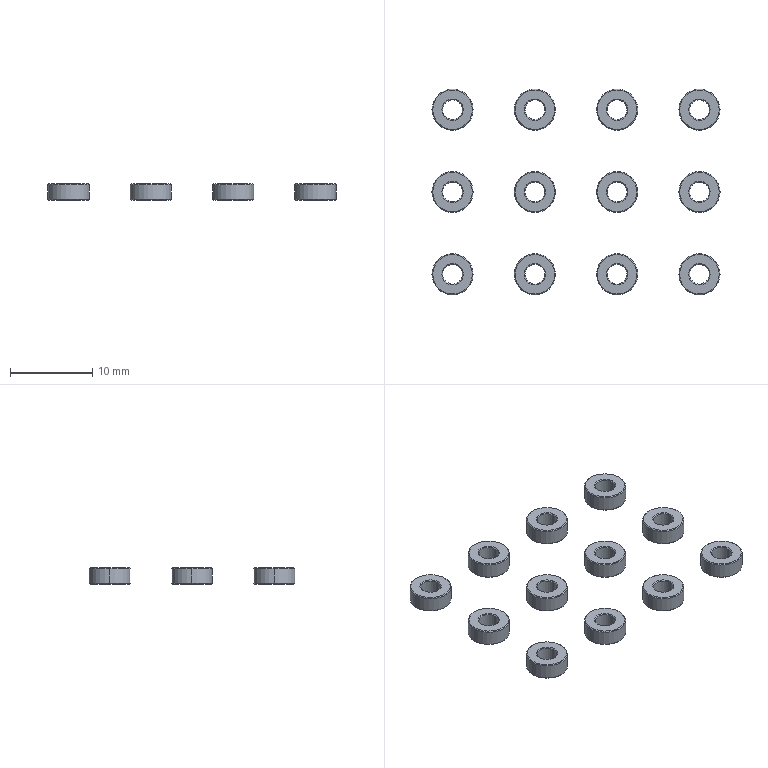NC program | NX | posted with a generic post | part box 35 x 25 x 2 mm
Lines 3718 to 5177 of 5177:
(ZLEVEL_PROFILE_1_COPY , TOOL : D6A45)
N7422 T07 M6
N7424 G54
N7426 G17 G0 G90 X2.2 Y22.5 S9500 M3
N7428 G43 Z30. H7
N7430 Z2.
N7432 G94 G1 Z-1. F1250.
N7434 G3 X2.5 Y22.2 R0.3
N7436 X2.2 Y22.5 R-0.3
N7438 X2.35 Y22.24 R0.3
N7440 G1 Z1.
N7442 G0 Z30.
N7444 X32.5 Y22.8
N7446 Z2.
N7448 G1 Z-1.
N7450 G3 X32.2 Y22.5 R0.3
N7452 X32.5 Y22.8 R-0.3
N7454 X32.24 Y22.65 R0.3
N7456 G1 Z1.
N7458 G0 Z30.
N7460 X22.5 Y22.8
N7462 Z2.
N7464 G1 Z-1.
N7466 G3 X22.2 Y22.5 R0.3
N7468 X22.5 Y22.8 R-0.3
N7470 X22.24 Y22.65 R0.3
N7472 G1 Z1.
N7474 G0 Z30.
N7476 X12.5 Y22.8
N7478 Z2.
N7480 G1 Z-1.
N7482 G3 X12.2 Y22.5 R0.3
N7484 X12.5 Y22.8 R-0.3
N7486 X12.24 Y22.65 R0.3
N7488 G1 Z1.
N7490 G0 Z30.
N7492 X32.8 Y12.5
N7494 Z2.
N7496 G1 Z-1.
N7498 Y12.512
N7500 G3 X32.8 Y12.5 R-0.3
N7502 X32.65 Y12.76 R0.3
N7504 G1 Z1.
N7506 G0 Z30.
N7508 X22.5 Y12.8
N7510 Z2.
N7512 G1 Z-1.
N7514 G3 X22.2 Y12.5 R0.3
N7516 X22.5 Y12.8 R-0.3
N7518 X22.24 Y12.65 R0.3
N7520 G1 Z1.
N7522 G0 Z30.
N7524 X12.5 Y12.2
N7526 Z2.
N7528 G1 Z-1.
N7530 G3 X12.8 Y12.5 R0.3
N7532 X12.5 Y12.2 R-0.3
N7534 X12.76 Y12.35 R0.3
N7536 G1 Z1.
N7538 G0 Z30.
N7540 X2.2 Y12.5
N7542 Z2.
N7544 G1 Z-1.
N7546 Y12.488
N7548 G3 X2.2 Y12.5 R-0.3
N7550 X2.35 Y12.24 R0.3
N7552 G1 Z1.
N7554 G0 Z30.
N7556 X32.5 Y2.2
N7558 Z2.
N7560 G1 Z-1.
N7562 G3 X32.8 Y2.5 R0.3
N7564 X32.5 Y2.2 R-0.3
N7566 X32.76 Y2.35 R0.3
N7568 G1 Z1.
N7570 G0 Z30.
N7572 X22.5 Y2.2
N7574 Z2.
N7576 G1 Z-1.
N7578 X22.553 Y2.205
N7580 G3 X22.5 Y2.2 R-0.3
N7582 X22.76 Y2.35 R0.3
N7584 G1 Z1.
N7586 G0 Z30.
N7588 X12.5 Y2.2
N7590 Z2.
N7592 G1 Z-1.
N7594 G3 X12.8 Y2.5 R0.3
N7596 X12.5 Y2.2 R-0.3
N7598 X12.76 Y2.35 R0.3
N7600 G1 Z1.
N7602 G0 Z30.
N7604 X2.5 Y2.2
N7606 Z2.
N7608 G1 Z-1.
N7610 G3 X2.8 Y2.5 R0.3
N7612 X2.5 Y2.2 R-0.3
N7614 X2.76 Y2.35 R0.3
N7616 G1 Z1.
N7618 G0 Z30.
N7620 X3.478 Y-1.995
N7622 Z1.
N7624 G1 Z-1.
N7626 X3.02 Y-1.2
N7628 G3 X2.5 Y-0.9 R0.6
N7630 G2 X-0.9 Y2.5 R3.4
N7632 X2.5 Y-0.9 R-3.4
N7634 G3 X1.98 Y-1.2 R0.6
N7636 G1 X1.522 Y-1.995
N7638 Z1.
N7640 G0 Z30.
N7642 X13.478
N7644 Z1.
N7646 G1 Z-1.
N7648 X13.02 Y-1.2
N7650 G3 X12.5 Y-0.9 R0.6
N7652 G2 X9.1 Y2.5 R3.4
N7654 X12.5 Y-0.9 R-3.4
N7656 G3 X11.98 Y-1.2 R0.6
N7658 G1 X11.522 Y-1.995
N7660 Z1.
N7662 G0 Z30.
N7664 X23.478
N7666 Z1.
N7668 G1 Z-1.
N7670 X23.02 Y-1.2
N7672 G3 X22.5 Y-0.9 R0.6
N7674 G2 X19.1 Y2.5 R3.4
N7676 X22.5 Y-0.9 R-3.4
N7678 G3 X21.98 Y-1.2 R0.6
N7680 G1 X21.522 Y-1.995
N7682 Z1.
N7684 G0 Z30.
N7686 X33.478
N7688 Z1.
N7690 G1 Z-1.
N7692 X33.02 Y-1.2
N7694 G3 X32.5 Y-0.9 R0.6
N7696 G2 X29.1 Y2.5 R3.4
N7698 X32.5 Y-0.9 R-3.4
N7700 G3 X31.98 Y-1.2 R0.6
N7702 G1 X31.522 Y-1.995
N7704 Z1.
N7706 G0 Z30.
N7708 X-1.995 Y11.522
N7710 Z1.
N7712 G1 Z-1.
N7714 X-1.2 Y11.98
N7716 G3 X-0.9 Y12.5 R0.6
N7718 G1 Y12.504
N7720 G2 X2.504 Y15.9 R3.4
N7722 X-0.9 Y12.5 R-3.4
N7724 G3 X-1.2 Y13.02 R0.6
N7726 G1 X-1.995 Y13.478
N7728 Z1.
N7730 G0 Z30.
N7732 X8.005 Y11.522
N7734 Z1.
N7736 G1 Z-1.
N7738 X8.8 Y11.98
N7740 G3 X9.1 Y12.5 R0.6
N7742 G2 X12.5 Y15.9 R3.4
N7744 X9.1 Y12.5 R-3.4
N7746 G3 X8.8 Y13.02 R0.6
N7748 G1 X8.005 Y13.478
N7750 Z1.
N7752 G0 Z30.
N7754 X21.522 Y16.995
N7756 Z1.
N7758 G1 Z-1.
N7760 X21.98 Y16.2
N7762 G3 X22.5 Y15.9 R0.6
N7764 G2 X25.9 Y12.5 R3.4
N7766 X22.5 Y15.9 R-3.4
N7768 G3 X23.02 Y16.2 R0.6
N7770 G1 X23.478 Y16.995
N7772 Z1.
N7774 G0 Z30.
N7776 X36.995 Y13.478
N7778 Z1.
N7780 G1 Z-1.
N7782 X36.2 Y13.02
N7784 G3 X35.9 Y12.5 R0.6
N7786 G1 Y12.496
N7788 G2 X32.496 Y9.1 R3.4
N7790 X35.9 Y12.5 R-3.4
N7792 G3 X36.2 Y11.98 R0.6
N7794 G1 X36.995 Y11.522
N7796 Z1.
N7798 G0 Z30.
N7800 X11.522 Y26.995
N7802 Z1.
N7804 G1 Z-1.
N7806 X11.98 Y26.2
N7808 G3 X12.5 Y25.9 R0.6
N7810 G2 X15.9 Y22.5 R3.4
N7812 X12.5 Y25.9 R-3.4
N7814 G3 X13.02 Y26.2 R0.6
N7816 G1 X13.478 Y26.995
N7818 Z1.
N7820 G0 Z30.
N7822 X21.522
N7824 Z1.
N7826 G1 Z-1.
N7828 X21.98 Y26.2
N7830 G3 X22.5 Y25.9 R0.6
N7832 G2 X25.9 Y22.5 R3.4
N7834 X22.5 Y25.9 R-3.4
N7836 G3 X23.02 Y26.2 R0.6
N7838 G1 X23.478 Y26.995
N7840 Z1.
N7842 G0 Z30.
N7844 X31.522
N7846 Z1.
N7848 G1 Z-1.
N7850 X31.98 Y26.2
N7852 G3 X32.5 Y25.9 R0.6
N7854 G2 X35.9 Y22.5 R3.4
N7856 X32.5 Y25.9 R-3.4
N7858 G3 X33.02 Y26.2 R0.6
N7860 G1 X33.478 Y26.995
N7862 Z1.
N7864 G0 Z30.
N7866 X1.522
N7868 Z1.
N7870 G1 Z-1.
N7872 X1.98 Y26.2
N7874 G3 X2.5 Y25.9 R0.6
N7876 G2 X5.9 Y22.5 R3.4
N7878 X2.5 Y25.9 R-3.4
N7880 G3 X3.02 Y26.2 R0.6
N7882 G1 X3.478 Y26.995
N7884 Z1.
N7886 G0 Z30.
N7888 M5
(ZLEVEL_PROFILE_COPY , TOOL : D4)
N7890 T04 M6
N7892 G54
N7894 G17 G0 G90 X36.171 Y15.114 S9500 M3
N7896 G43 Z30. H4
N7898 Z0.1
N7900 G94 G1 X36.688 Y14.227 Z0.046 F1000.
N7902 X36.998 Y13.036 Z-0.018
N7904 X37. Y12.5 Z-0.046
N7906 Y11.98 Z-0.074
N7908 X36.848 Y11.229 Z-0.114
N7910 X36.572 Y10.514 Z-0.154
N7912 X36.011 Y9.637 Z-0.208
N7914 X35.025 Y8.739 Z-0.278
N7916 X33.82 Y8.166 Z-0.348
N7918 X32.5 Y7.97 Z-0.418
N7920 X31.18 Y8.166 Z-0.488
N7922 X29.975 Y8.739 Z-0.558
N7924 X28.989 Y9.637 Z-0.628
N7926 X28.428 Y10.514 Z-0.683
N7928 X28.15 Y11.236 Z-0.723
N7930 X27.998 Y11.995 Z-0.764
N7932 X28.002 Y13.036 Z-0.818
N7934 X28.392 Y14.41 Z-0.893
N7936 X29.192 Y15.595 Z-0.968
N7938 X30.321 Y16.471 Z-1.043
N7940 X31.666 Y16.953 Z-1.118
N7942 X33.095 Y16.991 Z-1.193
N7944 X34.104 Y16.737 Z-1.247
N7946 X35.185 Y16.148 Z-1.312
N7948 X36.068 Y15.291 Z-1.376
N7950 X36.688 Y14.227 Z-1.441
N7952 X36.998 Y13.036 Z-1.505
N7954 X37. Y12.5 Z-1.533
N7956 G2 X32.5 Y8. R4.5
N7958 X37. Y12.5 R-4.5
N7960 G1 X36.994 Y12.261 Z-1.538
N7962 X36.975 Y12.023 Z-1.542
N7964 X36.943 Y11.787 Z-1.546
N7966 X36.899 Y11.552 Z-1.55
N7968 X36.843 Y11.32 Z-1.554
N7970 X36.774 Y11.092 Z-1.558
N7972 X36.693 Y10.867 Z-1.563
N7974 X36.601 Y10.647 Z-1.567
N7976 X36.497 Y10.432 Z-1.571
N7978 X36.382 Y10.223 Z-1.575
N7980 X36.255 Y10.021 Z-1.579
N7982 X36.119 Y9.825 Z-1.583
N7984 X35.972 Y9.637 Z-1.588
N7986 X35.815 Y9.457 Z-1.592
N7988 X35.649 Y9.285 Z-1.596
N7990 X35.474 Y9.123 Z-1.6
N7992 X35.291 Y8.97 Z-1.604
N7994 X35.1 Y8.827 Z-1.608
N7996 X34.901 Y8.694 Z-1.613
N7998 X34.696 Y8.572 Z-1.617
N8000 X34.485 Y8.461 Z-1.621
N8002 X34.268 Y8.362 Z-1.625
N8004 X34.046 Y8.274 Z-1.629
N8006 X33.82 Y8.198 Z-1.633
N8008 X33.59 Y8.134 Z-1.638
N8010 X33.357 Y8.082 Z-1.642
N8012 X33.121 Y8.043 Z-1.646
N8014 X32.884 Y8.016 Z-1.65
N8016 X32.646 Y8.002 Z-1.654
N8018 X32.407 Y8.001 Z-1.658
N8020 X32.169 Y8.012 Z-1.663
N8022 X31.931 Y8.036 Z-1.667
N8024 G2 X37. Y12.5 R-4.5
N8026 G1 X36.994 Y12.261 Z-1.671
N8028 X36.975 Y12.023 Z-1.675
N8030 X36.943 Y11.787 Z-1.679
N8032 X36.899 Y11.552 Z-1.683
N8034 X36.843 Y11.32 Z-1.688
N8036 X36.774 Y11.092 Z-1.692
N8038 X36.693 Y10.867 Z-1.696
N8040 X36.601 Y10.647 Z-1.7
N8042 X36.497 Y10.432 Z-1.704
N8044 X36.382 Y10.223 Z-1.708
N8046 X36.255 Y10.021 Z-1.713
N8048 X36.119 Y9.825 Z-1.717
N8050 X35.972 Y9.637 Z-1.721
N8052 X35.815 Y9.457 Z-1.725
N8054 X35.649 Y9.285 Z-1.729
N8056 X35.474 Y9.123 Z-1.733
N8058 X35.291 Y8.97 Z-1.738
N8060 X35.1 Y8.827 Z-1.742
N8062 X34.901 Y8.694 Z-1.746
N8064 X34.696 Y8.572 Z-1.75
N8066 X34.485 Y8.461 Z-1.754
N8068 X34.268 Y8.362 Z-1.758
N8070 X34.046 Y8.274 Z-1.763
N8072 X33.82 Y8.198 Z-1.767
N8074 X33.59 Y8.134 Z-1.771
N8076 X33.357 Y8.082 Z-1.775
N8078 X33.121 Y8.043 Z-1.779
N8080 X32.884 Y8.016 Z-1.783
N8082 X32.646 Y8.002 Z-1.788
N8084 X32.407 Y8.001 Z-1.792
N8086 X32.169 Y8.012 Z-1.796
N8088 X31.931 Y8.036 Z-1.8
N8090 G2 X28.036 Y13.069 R4.5
N8092 X31.931 Y8.036 R-4.5
N8094 G1 Z-0.3
N8096 G0 Z53.
N8098 X5.115 Y-1.192
N8100 Z0.1
N8102 G1 X4.141 Y-1.722 Z0.042
N8104 X3.02 Y-2. Z-0.019
N8106 X1.98 Z-0.073
N8108 X0.921 Y-1.746 Z-0.13
N8110 X-0.046 Y-1.247 Z-0.187
N8112 X-0.867 Y-0.531 Z-0.244
N8114 X-1.47 Y0.318 Z-0.299
N8116 X-1.818 Y1.13 Z-0.345
N8118 X-2.002 Y1.994 Z-0.392
N8120 X-1.998 Y3.035 Z-0.446
N8122 X-1.665 Y4.282 Z-0.514
N8124 X-0.993 Y5.385 Z-0.581
N8126 X-0.037 Y6.253 Z-0.649
N8128 X1.124 Y6.816 Z-0.717
N8130 X2.397 Y7.029 Z-0.784
N8132 X3.679 Y6.874 Z-0.852
N8134 X4.646 Y6.489 Z-0.907
N8136 X5.791 Y5.613 Z-0.982
N8138 X6.602 Y4.421 Z-1.058
N8140 X6.998 Y3.035 Z-1.133
N8142 X7.002 Y1.994 Z-1.188
N8144 X6.847 Y1.226 Z-1.229
N8146 X6.562 Y0.495 Z-1.27
N8148 X5.997 Y-0.379 Z-1.324
N8150 X5.156 Y-1.17 Z-1.385
N8152 X4.141 Y-1.722 Z-1.446
N8154 X3.02 Y-2. Z-1.506
N8156 X2.5 Z-1.533
N8158 G2 X-2. Y2.5 R4.5
N8160 X2.5 Y-2. R-4.5
N8162 G1 X2.261 Y-1.994 Z-1.538
N8164 X2.023 Y-1.975 Z-1.542
N8166 X1.787 Y-1.943 Z-1.546
N8168 X1.552 Y-1.899 Z-1.55
N8170 X1.32 Y-1.843 Z-1.554
N8172 X1.092 Y-1.774 Z-1.558
N8174 X0.867 Y-1.693 Z-1.563
N8176 X0.647 Y-1.601 Z-1.567
N8178 X0.432 Y-1.497 Z-1.571
N8180 X0.223 Y-1.382 Z-1.575
N8182 X0.021 Y-1.255 Z-1.579
N8184 X-0.175 Y-1.119 Z-1.583
N8186 X-0.363 Y-0.972 Z-1.588
N8188 X-0.543 Y-0.815 Z-1.592
N8190 X-0.715 Y-0.649 Z-1.596
N8192 X-0.877 Y-0.474 Z-1.6
N8194 X-1.03 Y-0.291 Z-1.604
N8196 X-1.173 Y-0.1 Z-1.608
N8198 X-1.306 Y0.099 Z-1.613
N8200 X-1.428 Y0.304 Z-1.617
N8202 X-1.539 Y0.515 Z-1.621
N8204 X-1.638 Y0.732 Z-1.625
N8206 X-1.726 Y0.954 Z-1.629
N8208 X-1.802 Y1.18 Z-1.633
N8210 X-1.866 Y1.41 Z-1.638
N8212 X-1.918 Y1.643 Z-1.642
N8214 X-1.957 Y1.879 Z-1.646
N8216 X-1.984 Y2.116 Z-1.65
N8218 X-1.998 Y2.354 Z-1.654
N8220 X-1.999 Y2.593 Z-1.658
N8222 X-1.988 Y2.831 Z-1.663
N8224 X-1.964 Y3.069 Z-1.667
N8226 G2 X2.5 Y-2. R-4.5
N8228 G1 X2.261 Y-1.994 Z-1.671
N8230 X2.023 Y-1.975 Z-1.675
N8232 X1.787 Y-1.943 Z-1.679
N8234 X1.552 Y-1.899 Z-1.683
N8236 X1.32 Y-1.843 Z-1.688
N8238 X1.092 Y-1.774 Z-1.692
N8240 X0.867 Y-1.693 Z-1.696
N8242 X0.647 Y-1.601 Z-1.7
N8244 X0.432 Y-1.497 Z-1.704
N8246 X0.223 Y-1.382 Z-1.708
N8248 X0.021 Y-1.255 Z-1.713
N8250 X-0.175 Y-1.119 Z-1.717
N8252 X-0.363 Y-0.972 Z-1.721
N8254 X-0.543 Y-0.815 Z-1.725
N8256 X-0.715 Y-0.649 Z-1.729
N8258 X-0.877 Y-0.474 Z-1.733
N8260 X-1.03 Y-0.291 Z-1.738
N8262 X-1.173 Y-0.1 Z-1.742
N8264 X-1.306 Y0.099 Z-1.746
N8266 X-1.428 Y0.304 Z-1.75
N8268 X-1.539 Y0.515 Z-1.754
N8270 X-1.638 Y0.732 Z-1.758
N8272 X-1.726 Y0.954 Z-1.763
N8274 X-1.802 Y1.18 Z-1.767
N8276 X-1.866 Y1.41 Z-1.771
N8278 X-1.918 Y1.643 Z-1.775
N8280 X-1.957 Y1.879 Z-1.779
N8282 X-1.984 Y2.116 Z-1.783
N8284 X-1.998 Y2.354 Z-1.788
N8286 X-1.999 Y2.593 Z-1.792
N8288 X-1.988 Y2.831 Z-1.796
N8290 X-1.964 Y3.069 Z-1.8
N8292 G2 X3.069 Y6.964 R4.5
N8294 X-1.964 Y3.069 R-4.5
N8296 G1 Z-0.3
N8298 G0 Z53.
N8300 X9.888 Y26.178
N8302 Z0.1
N8304 G1 X10.803 Y26.7 Z0.045
N8306 X11.98 Y27. Z-0.019
N8308 X13.02 Z-0.073
N8310 X13.968 Y26.785 Z-0.124
N8312 X14.908 Y26.337 Z-0.179
N8314 X15.933 Y25.456 Z-0.25
N8316 X16.652 Y24.311 Z-0.321
N8318 X17.002 Y23.006 Z-0.391
N8320 X16.998 Y21.965 Z-0.446
N8322 X16.79 Y21.044 Z-0.495
N8324 X16.395 Y20.187 Z-0.545
N8326 X15.764 Y19.359 Z-0.599
N8328 X14.731 Y18.557 Z-0.668
N8330 X13.511 Y18.084 Z-0.737
N8332 X12.207 Y17.979 Z-0.805
N8334 X10.928 Y18.252 Z-0.874
N8336 X9.779 Y18.878 Z-0.942
N8338 X8.858 Y19.807 Z-1.011
N8340 X8.339 Y20.709 Z-1.065
N8342 X8.002 Y21.965 Z-1.133
N8344 X7.998 Y23.006 Z-1.188
N8346 X8.294 Y24.183 Z-1.252
N8348 X8.892 Y25.239 Z-1.315
N8350 X9.749 Y26.099 Z-1.379
N8352 X10.803 Y26.7 Z-1.442
N8354 X11.98 Y27. Z-1.506
N8356 X12.5 Z-1.533
N8358 G2 X17. Y22.5 R4.5
N8360 X12.5 Y27. R-4.5
N8362 G1 X12.739 Y26.994 Z-1.538
N8364 X12.977 Y26.975 Z-1.542
N8366 X13.213 Y26.943 Z-1.546
N8368 X13.448 Y26.899 Z-1.55
N8370 X13.68 Y26.843 Z-1.554
N8372 X13.908 Y26.774 Z-1.558
N8374 X14.133 Y26.693 Z-1.563
N8376 X14.353 Y26.601 Z-1.567
N8378 X14.568 Y26.497 Z-1.571
N8380 X14.777 Y26.382 Z-1.575
N8382 X14.979 Y26.255 Z-1.579
N8384 X15.175 Y26.119 Z-1.583
N8386 X15.363 Y25.972 Z-1.588
N8388 X15.543 Y25.815 Z-1.592
N8390 X15.715 Y25.649 Z-1.596
N8392 X15.877 Y25.474 Z-1.6
N8394 X16.03 Y25.291 Z-1.604
N8396 X16.173 Y25.1 Z-1.608
N8398 X16.306 Y24.901 Z-1.613
N8400 X16.428 Y24.696 Z-1.617
N8402 X16.539 Y24.485 Z-1.621
N8404 X16.638 Y24.268 Z-1.625
N8406 X16.726 Y24.046 Z-1.629
N8408 X16.802 Y23.82 Z-1.633
N8410 X16.866 Y23.59 Z-1.638
N8412 X16.918 Y23.357 Z-1.642
N8414 X16.957 Y23.121 Z-1.646
N8416 X16.984 Y22.884 Z-1.65
N8418 X16.998 Y22.646 Z-1.654
N8420 X16.999 Y22.407 Z-1.658
N8422 X16.988 Y22.169 Z-1.663
N8424 X16.964 Y21.931 Z-1.667
N8426 G2 X12.5 Y27. R-4.5
N8428 G1 X12.739 Y26.994 Z-1.671
N8430 X12.977 Y26.975 Z-1.675
N8432 X13.213 Y26.943 Z-1.679
N8434 X13.448 Y26.899 Z-1.683
N8436 X13.68 Y26.843 Z-1.688
N8438 X13.908 Y26.774 Z-1.692
N8440 X14.133 Y26.693 Z-1.696
N8442 X14.353 Y26.601 Z-1.7
N8444 X14.568 Y26.497 Z-1.704
N8446 X14.777 Y26.382 Z-1.708
N8448 X14.979 Y26.255 Z-1.713
N8450 X15.175 Y26.119 Z-1.717
N8452 X15.363 Y25.972 Z-1.721
N8454 X15.543 Y25.815 Z-1.725
N8456 X15.715 Y25.649 Z-1.729
N8458 X15.877 Y25.474 Z-1.733
N8460 X16.03 Y25.291 Z-1.738
N8462 X16.173 Y25.1 Z-1.742
N8464 X16.306 Y24.901 Z-1.746
N8466 X16.428 Y24.696 Z-1.75
N8468 X16.539 Y24.485 Z-1.754
N8470 X16.638 Y24.268 Z-1.758
N8472 X16.726 Y24.046 Z-1.763
N8474 X16.802 Y23.82 Z-1.767
N8476 X16.866 Y23.59 Z-1.771
N8478 X16.918 Y23.357 Z-1.775
N8480 X16.957 Y23.121 Z-1.779
N8482 X16.984 Y22.884 Z-1.783
N8484 X16.998 Y22.646 Z-1.788
N8486 X16.999 Y22.407 Z-1.792
N8488 X16.988 Y22.169 Z-1.796
N8490 X16.964 Y21.931 Z-1.8
N8492 G2 X11.931 Y18.036 R4.5
N8494 X16.964 Y21.931 R-4.5
N8496 G1 Z-0.3
N8498 G0 Z53.
N8500 X15.111 Y-1.19
N8502 Z0.1
N8504 G1 X15.046 Y-1.247 Z0.096
N8506 X14.079 Y-1.746 Z0.038
N8508 X13.02 Y-2. Z-0.019
N8510 X11.98 Z-0.073
N8512 X10.921 Y-1.746 Z-0.13
N8514 X9.954 Y-1.247 Z-0.187
N8516 X9.133 Y-0.531 Z-0.244
N8518 X8.53 Y0.318 Z-0.299
N8520 X8.182 Y1.13 Z-0.345
N8522 X7.998 Y1.994 Z-0.391
N8524 X8.002 Y3.035 Z-0.446
N8526 X8.335 Y4.282 Z-0.514
N8528 X9.007 Y5.385 Z-0.581
N8530 X9.963 Y6.253 Z-0.649
N8532 X11.124 Y6.816 Z-0.717
N8534 X12.397 Y7.029 Z-0.784
N8536 X13.679 Y6.874 Z-0.852
N8538 X14.646 Y6.489 Z-0.907
N8540 X15.791 Y5.613 Z-0.982
N8542 X16.602 Y4.421 Z-1.058
N8544 X16.998 Y3.035 Z-1.133
N8546 X17.002 Y1.994 Z-1.188
N8548 X16.818 Y1.13 Z-1.234
N8550 X16.47 Y0.318 Z-1.28
N8552 X15.867 Y-0.531 Z-1.335
N8554 X15.046 Y-1.247 Z-1.392
N8556 X14.079 Y-1.746 Z-1.449
N8558 X13.02 Y-2. Z-1.506
N8560 X12.5 Z-1.533
N8562 G2 X8. Y2.5 R4.5
N8564 X12.5 Y-2. R-4.5
N8566 G1 X12.261 Y-1.994 Z-1.538
N8568 X12.023 Y-1.975 Z-1.542
N8570 X11.787 Y-1.943 Z-1.546
N8572 X11.552 Y-1.899 Z-1.55
N8574 X11.32 Y-1.843 Z-1.554
N8576 X11.092 Y-1.774 Z-1.558
N8578 X10.867 Y-1.693 Z-1.563
N8580 X10.647 Y-1.601 Z-1.567
N8582 X10.432 Y-1.497 Z-1.571
N8584 X10.223 Y-1.382 Z-1.575
N8586 X10.021 Y-1.255 Z-1.579
N8588 X9.825 Y-1.119 Z-1.583
N8590 X9.637 Y-0.972 Z-1.588
N8592 X9.457 Y-0.815 Z-1.592
N8594 X9.285 Y-0.649 Z-1.596
N8596 X9.123 Y-0.474 Z-1.6
N8598 X8.97 Y-0.291 Z-1.604
N8600 X8.827 Y-0.1 Z-1.608
N8602 X8.694 Y0.099 Z-1.613
N8604 X8.572 Y0.304 Z-1.617
N8606 X8.461 Y0.515 Z-1.621
N8608 X8.362 Y0.732 Z-1.625
N8610 X8.274 Y0.954 Z-1.629
N8612 X8.198 Y1.18 Z-1.633
N8614 X8.134 Y1.41 Z-1.638
N8616 X8.082 Y1.643 Z-1.642
N8618 X8.043 Y1.879 Z-1.646
N8620 X8.016 Y2.116 Z-1.65
N8622 X8.002 Y2.354 Z-1.654
N8624 X8.001 Y2.593 Z-1.658
N8626 X8.012 Y2.831 Z-1.663
N8628 X8.036 Y3.069 Z-1.667
N8630 G2 X12.5 Y-2. R-4.5
N8632 G1 X12.261 Y-1.994 Z-1.671
N8634 X12.023 Y-1.975 Z-1.675
N8636 X11.787 Y-1.943 Z-1.679
N8638 X11.552 Y-1.899 Z-1.683
N8640 X11.32 Y-1.843 Z-1.688
N8642 X11.092 Y-1.774 Z-1.692
N8644 X10.867 Y-1.693 Z-1.696
N8646 X10.647 Y-1.601 Z-1.7
N8648 X10.432 Y-1.497 Z-1.704
N8650 X10.223 Y-1.382 Z-1.708
N8652 X10.021 Y-1.255 Z-1.713
N8654 X9.825 Y-1.119 Z-1.717
N8656 X9.637 Y-0.972 Z-1.721
N8658 X9.457 Y-0.815 Z-1.725
N8660 X9.285 Y-0.649 Z-1.729
N8662 X9.123 Y-0.474 Z-1.733
N8664 X8.97 Y-0.291 Z-1.738
N8666 X8.827 Y-0.1 Z-1.742
N8668 X8.694 Y0.099 Z-1.746
N8670 X8.572 Y0.304 Z-1.75
N8672 X8.461 Y0.515 Z-1.754
N8674 X8.362 Y0.732 Z-1.758
N8676 X8.274 Y0.954 Z-1.763
N8678 X8.198 Y1.18 Z-1.767
N8680 X8.134 Y1.41 Z-1.771
N8682 X8.082 Y1.643 Z-1.775
N8684 X8.043 Y1.879 Z-1.779
N8686 X8.016 Y2.116 Z-1.783
N8688 X8.002 Y2.354 Z-1.788
N8690 X8.001 Y2.593 Z-1.792
N8692 X8.012 Y2.831 Z-1.796
N8694 X8.036 Y3.069 Z-1.8
N8696 G2 X13.069 Y6.964 R4.5
N8698 X8.036 Y3.069 R-4.5
N8700 G1 Z-0.3
N8702 G0 Z53.
N8704 X25.115 Y-1.192
N8706 Z0.1
N8708 G1 X24.142 Y-1.722 Z0.042
N8710 X23.02 Y-2. Z-0.019
N8712 X21.98 Z-0.073
N8714 X20.921 Y-1.746 Z-0.13
N8716 X19.954 Y-1.247 Z-0.187
N8718 X19.133 Y-0.531 Z-0.244
N8720 X18.53 Y0.318 Z-0.299
N8722 X18.182 Y1.13 Z-0.345
N8724 X17.998 Y1.994 Z-0.392
N8726 X18.002 Y3.035 Z-0.446
N8728 X18.335 Y4.282 Z-0.514
N8730 X19.007 Y5.385 Z-0.581
N8732 X19.963 Y6.253 Z-0.649
N8734 X21.124 Y6.816 Z-0.717
N8736 X22.397 Y7.029 Z-0.784
N8738 X23.679 Y6.874 Z-0.852
N8740 X24.646 Y6.489 Z-0.907
N8742 X25.791 Y5.613 Z-0.982
N8744 X26.602 Y4.421 Z-1.058
N8746 X26.998 Y3.035 Z-1.133
N8748 X27.002 Y1.994 Z-1.188
N8750 X26.847 Y1.227 Z-1.229
N8752 X26.563 Y0.497 Z-1.27
N8754 X25.999 Y-0.377 Z-1.324
N8756 X25.157 Y-1.169 Z-1.385
N8758 X24.142 Y-1.722 Z-1.445
N8760 X23.02 Y-2. Z-1.506
N8762 X22.5 Z-1.533
N8764 G2 X18. Y2.5 R4.5
N8766 X22.5 Y-2. R-4.5
N8768 G1 X22.261 Y-1.994 Z-1.538
N8770 X22.023 Y-1.975 Z-1.542
N8772 X21.787 Y-1.943 Z-1.546
N8774 X21.552 Y-1.899 Z-1.55
N8776 X21.32 Y-1.843 Z-1.554
N8778 X21.092 Y-1.774 Z-1.558
N8780 X20.867 Y-1.693 Z-1.563
N8782 X20.647 Y-1.601 Z-1.567
N8784 X20.432 Y-1.497 Z-1.571
N8786 X20.223 Y-1.382 Z-1.575
N8788 X20.021 Y-1.255 Z-1.579
N8790 X19.825 Y-1.119 Z-1.583
N8792 X19.637 Y-0.972 Z-1.588
N8794 X19.457 Y-0.815 Z-1.592
N8796 X19.285 Y-0.649 Z-1.596
N8798 X19.123 Y-0.474 Z-1.6
N8800 X18.97 Y-0.291 Z-1.604
N8802 X18.827 Y-0.1 Z-1.608
N8804 X18.694 Y0.099 Z-1.613
N8806 X18.572 Y0.304 Z-1.617
N8808 X18.461 Y0.515 Z-1.621
N8810 X18.362 Y0.732 Z-1.625
N8812 X18.274 Y0.954 Z-1.629
N8814 X18.198 Y1.18 Z-1.633
N8816 X18.134 Y1.41 Z-1.638
N8818 X18.082 Y1.643 Z-1.642
N8820 X18.043 Y1.879 Z-1.646
N8822 X18.016 Y2.116 Z-1.65
N8824 X18.002 Y2.354 Z-1.654
N8826 X18.001 Y2.593 Z-1.658
N8828 X18.012 Y2.831 Z-1.663
N8830 X18.036 Y3.069 Z-1.667
N8832 G2 X22.5 Y-2. R-4.5
N8834 G1 X22.261 Y-1.994 Z-1.671
N8836 X22.023 Y-1.975 Z-1.675
N8838 X21.787 Y-1.943 Z-1.679
N8840 X21.552 Y-1.899 Z-1.683
N8842 X21.32 Y-1.843 Z-1.688
N8844 X21.092 Y-1.774 Z-1.692
N8846 X20.867 Y-1.693 Z-1.696
N8848 X20.647 Y-1.601 Z-1.7
N8850 X20.432 Y-1.497 Z-1.704
N8852 X20.223 Y-1.382 Z-1.708
N8854 X20.021 Y-1.255 Z-1.713
N8856 X19.825 Y-1.119 Z-1.717
N8858 X19.637 Y-0.972 Z-1.721
N8860 X19.457 Y-0.815 Z-1.725
N8862 X19.285 Y-0.649 Z-1.729
N8864 X19.123 Y-0.474 Z-1.733
N8866 X18.97 Y-0.291 Z-1.738
N8868 X18.827 Y-0.1 Z-1.742
N8870 X18.694 Y0.099 Z-1.746
N8872 X18.572 Y0.304 Z-1.75
N8874 X18.461 Y0.515 Z-1.754
N8876 X18.362 Y0.732 Z-1.758
N8878 X18.274 Y0.954 Z-1.763
N8880 X18.198 Y1.18 Z-1.767
N8882 X18.134 Y1.41 Z-1.771
N8884 X18.082 Y1.643 Z-1.775
N8886 X18.043 Y1.879 Z-1.779
N8888 X18.016 Y2.116 Z-1.783
N8890 X18.002 Y2.354 Z-1.788
N8892 X18.001 Y2.593 Z-1.792
N8894 X18.012 Y2.831 Z-1.796
N8896 X18.036 Y3.069 Z-1.8
N8898 G2 X23.069 Y6.964 R4.5
N8900 X18.036 Y3.069 R-4.5
N8902 G1 Z-0.3
N8904 G0 Z53.
N8906 X36.153 Y25.105
N8908 Z0.1
N8910 G1 X36.648 Y24.32 Z0.051
N8912 X37. Y23.02 Z-0.019
N8914 Y22.485 Z-0.047
N8916 X36.998 Y21.965 Z-0.075
N8918 X36.79 Y21.044 Z-0.124
N8920 X36.395 Y20.187 Z-0.173
N8922 X35.764 Y19.359 Z-0.228
N8924 X34.731 Y18.557 Z-0.297
N8926 X33.511 Y18.084 Z-0.365
N8928 X32.207 Y17.979 Z-0.434
N8930 X30.928 Y18.252 Z-0.502
N8932 X29.779 Y18.878 Z-0.571
N8934 X28.858 Y19.807 Z-0.639
N8936 X28.339 Y20.709 Z-0.694
N8938 X28.002 Y21.965 Z-0.762
N8940 X27.998 Y23.006 Z-0.817
N8942 X28.346 Y24.306 Z-0.887
N8944 X29.059 Y25.447 Z-0.958
N8946 X30.077 Y26.327 Z-1.028
N8948 X31.308 Y26.87 Z-1.099
N8950 X32.645 Y27.028 Z-1.169
N8952 X33.968 Y26.785 Z-1.24
N8954 X34.908 Y26.337 Z-1.294
N8956 X35.93 Y25.46 Z-1.365
N8958 X36.648 Y24.32 Z-1.435
N8960 X37. Y23.02 Z-1.506
N8962 Y22.5 Z-1.533
N8964 Y22.485
N8966 G2 X32.485 Y18. R4.5
N8968 X37. Y22.5 R-4.5
N8970 G1 X36.994 Y22.261 Z-1.538
N8972 X36.975 Y22.023 Z-1.542
N8974 X36.943 Y21.787 Z-1.546
N8976 X36.899 Y21.552 Z-1.55
N8978 X36.843 Y21.32 Z-1.554
N8980 X36.774 Y21.092 Z-1.558
N8982 X36.693 Y20.867 Z-1.563
N8984 X36.601 Y20.647 Z-1.567
N8986 X36.497 Y20.432 Z-1.571
N8988 X36.382 Y20.223 Z-1.575
N8990 X36.255 Y20.021 Z-1.579
N8992 X36.119 Y19.825 Z-1.583
N8994 X35.972 Y19.637 Z-1.588
N8996 X35.815 Y19.457 Z-1.592
N8998 X35.649 Y19.285 Z-1.596
N9000 X35.474 Y19.123 Z-1.6
N9002 X35.291 Y18.97 Z-1.604
N9004 X35.1 Y18.827 Z-1.608
N9006 X34.901 Y18.694 Z-1.613
N9008 X34.696 Y18.572 Z-1.617
N9010 X34.485 Y18.461 Z-1.621
N9012 X34.268 Y18.362 Z-1.625
N9014 X34.046 Y18.274 Z-1.629
N9016 X33.82 Y18.198 Z-1.633
N9018 X33.59 Y18.134 Z-1.638
N9020 X33.357 Y18.082 Z-1.642
N9022 X33.121 Y18.043 Z-1.646
N9024 X32.884 Y18.016 Z-1.65
N9026 X32.646 Y18.002 Z-1.654
N9028 X32.407 Y18.001 Z-1.658
N9030 X32.169 Y18.012 Z-1.663
N9032 X31.931 Y18.036 Z-1.667
N9034 G2 X37. Y22.5 R-4.5
N9036 G1 X36.994 Y22.261 Z-1.671
N9038 X36.975 Y22.023 Z-1.675
N9040 X36.943 Y21.787 Z-1.679
N9042 X36.899 Y21.552 Z-1.683
N9044 X36.843 Y21.32 Z-1.688
N9046 X36.774 Y21.092 Z-1.692
N9048 X36.693 Y20.867 Z-1.696
N9050 X36.601 Y20.647 Z-1.7
N9052 X36.497 Y20.432 Z-1.704
N9054 X36.382 Y20.223 Z-1.708
N9056 X36.255 Y20.021 Z-1.713
N9058 X36.119 Y19.825 Z-1.717
N9060 X35.972 Y19.637 Z-1.721
N9062 X35.815 Y19.457 Z-1.725
N9064 X35.649 Y19.285 Z-1.729
N9066 X35.474 Y19.123 Z-1.733
N9068 X35.291 Y18.97 Z-1.738
N9070 X35.1 Y18.827 Z-1.742
N9072 X34.901 Y18.694 Z-1.746
N9074 X34.696 Y18.572 Z-1.75
N9076 X34.485 Y18.461 Z-1.754
N9078 X34.268 Y18.362 Z-1.758
N9080 X34.046 Y18.274 Z-1.763
N9082 X33.82 Y18.198 Z-1.767
N9084 X33.59 Y18.134 Z-1.771
N9086 X33.357 Y18.082 Z-1.775
N9088 X33.121 Y18.043 Z-1.779
N9090 X32.884 Y18.016 Z-1.783
N9092 X32.646 Y18.002 Z-1.788
N9094 X32.407 Y18.001 Z-1.792
N9096 X32.169 Y18.012 Z-1.796
N9098 X31.931 Y18.036 Z-1.8
N9100 G2 X28.036 Y23.069 R4.5
N9102 X31.931 Y18.036 R-4.5
N9104 G1 Z-0.3
N9106 G0 Z53.
N9108 X36.145 Y5.093
N9110 Z0.1
N9112 G1 X36.602 Y4.421 Z0.057
N9114 X36.998 Y3.035 Z-0.018
N9116 X37. Y2.5 Z-0.046
N9118 Y1.98 Z-0.073
N9120 X36.816 Y1.123 Z-0.119
N9122 X36.47 Y0.318 Z-0.165
N9124 X35.867 Y-0.531 Z-0.22
N9126 X34.901 Y-1.342 Z-0.286
N9128 X33.749 Y-1.854 Z-0.352
N9130 X32.5 Y-2.03 Z-0.418
N9132 X31.251 Y-1.854 Z-0.484
N9134 X30.099 Y-1.342 Z-0.55
N9136 X29.133 Y-0.531 Z-0.616
N9138 X28.53 Y0.318 Z-0.671
N9140 X28.182 Y1.13 Z-0.717
N9142 X27.998 Y1.994 Z-0.764
N9144 X28.002 Y3.035 Z-0.818
N9146 X28.335 Y4.282 Z-0.886
N9148 X29.007 Y5.385 Z-0.953
N9150 X29.963 Y6.253 Z-1.021
N9152 X31.124 Y6.816 Z-1.089
N9154 X32.397 Y7.029 Z-1.156
N9156 X33.679 Y6.874 Z-1.224
N9158 X34.646 Y6.489 Z-1.279
N9160 X35.791 Y5.613 Z-1.354
N9162 X36.602 Y4.421 Z-1.43
N9164 X36.998 Y3.035 Z-1.505
N9166 X37. Y2.5 Z-1.533
N9168 G2 X32.5 Y-2. R4.5
N9170 X37. Y2.5 R-4.5
N9172 G1 X36.994 Y2.261 Z-1.538
N9174 X36.975 Y2.023 Z-1.542
N9176 X36.943 Y1.787 Z-1.546
N9178 X36.899 Y1.552 Z-1.55
N9180 X36.843 Y1.32 Z-1.554
N9182 X36.774 Y1.092 Z-1.558
N9184 X36.693 Y0.867 Z-1.563
N9186 X36.601 Y0.647 Z-1.567
N9188 X36.497 Y0.432 Z-1.571
N9190 X36.382 Y0.223 Z-1.575
N9192 X36.255 Y0.021 Z-1.579
N9194 X36.119 Y-0.175 Z-1.583
N9196 X35.972 Y-0.363 Z-1.588
N9198 X35.815 Y-0.543 Z-1.592
N9200 X35.649 Y-0.715 Z-1.596
N9202 X35.474 Y-0.877 Z-1.6
N9204 X35.291 Y-1.03 Z-1.604
N9206 X35.1 Y-1.173 Z-1.608
N9208 X34.901 Y-1.306 Z-1.613
N9210 X34.696 Y-1.428 Z-1.617
N9212 X34.485 Y-1.539 Z-1.621
N9214 X34.268 Y-1.638 Z-1.625
N9216 X34.046 Y-1.726 Z-1.629
N9218 X33.82 Y-1.802 Z-1.633
N9220 X33.59 Y-1.866 Z-1.638
N9222 X33.357 Y-1.918 Z-1.642
N9224 X33.121 Y-1.957 Z-1.646
N9226 X32.884 Y-1.984 Z-1.65
N9228 X32.646 Y-1.998 Z-1.654
N9230 X32.407 Y-1.999 Z-1.658
N9232 X32.169 Y-1.988 Z-1.663
N9234 X31.931 Y-1.964 Z-1.667
N9236 G2 X37. Y2.5 R-4.5
N9238 G1 X36.994 Y2.261 Z-1.671
N9240 X36.975 Y2.023 Z-1.675
N9242 X36.943 Y1.787 Z-1.679
N9244 X36.899 Y1.552 Z-1.683
N9246 X36.843 Y1.32 Z-1.688
N9248 X36.774 Y1.092 Z-1.692
N9250 X36.693 Y0.867 Z-1.696
N9252 X36.601 Y0.647 Z-1.7
N9254 X36.497 Y0.432 Z-1.704
N9256 X36.382 Y0.223 Z-1.708
N9258 X36.255 Y0.021 Z-1.713
N9260 X36.119 Y-0.175 Z-1.717
N9262 X35.972 Y-0.363 Z-1.721
N9264 X35.815 Y-0.543 Z-1.725
N9266 X35.649 Y-0.715 Z-1.729
N9268 X35.474 Y-0.877 Z-1.733
N9270 X35.291 Y-1.03 Z-1.738
N9272 X35.1 Y-1.173 Z-1.742
N9274 X34.901 Y-1.306 Z-1.746
N9276 X34.696 Y-1.428 Z-1.75
N9278 X34.485 Y-1.539 Z-1.754
N9280 X34.268 Y-1.638 Z-1.758
N9282 X34.046 Y-1.726 Z-1.763
N9284 X33.82 Y-1.802 Z-1.767
N9286 X33.59 Y-1.866 Z-1.771
N9288 X33.357 Y-1.918 Z-1.775
N9290 X33.121 Y-1.957 Z-1.779
N9292 X32.884 Y-1.984 Z-1.783
N9294 X32.646 Y-1.998 Z-1.788
N9296 X32.407 Y-1.999 Z-1.792
N9298 X32.169 Y-1.988 Z-1.796
N9300 X31.931 Y-1.964 Z-1.8
N9302 G2 X28.036 Y3.069 R4.5
N9304 X31.931 Y-1.964 R-4.5
N9306 G1 Z-0.3
N9308 G0 Z53.
N9310 X-1.173 Y9.891
N9312 Z0.1
N9314 G1 X-1.572 Y10.514 Z0.061
N9316 X-1.848 Y11.229 Z0.021
N9318 X-2. Y11.98 Z-0.019
N9320 Y12.515 Z-0.047
N9322 X-1.998 Y13.036 Z-0.074
N9324 X-1.608 Y14.41 Z-0.149
N9326 X-0.808 Y15.595 Z-0.224
N9328 X0.32 Y16.471 Z-0.299
N9330 X1.666 Y16.952 Z-0.374
N9332 X3.094 Y16.991 Z-0.449
N9334 X4.103 Y16.737 Z-0.503
N9336 X5.185 Y16.149 Z-0.568
N9338 X6.068 Y15.291 Z-0.632
N9340 X6.688 Y14.227 Z-0.697
N9342 X6.998 Y13.036 Z-0.762
N9344 X7.002 Y11.995 Z-0.816
N9346 X6.85 Y11.236 Z-0.857
N9348 X6.572 Y10.514 Z-0.897
N9350 X6.011 Y9.637 Z-0.952
N9352 X5.025 Y8.739 Z-1.022
N9354 X3.82 Y8.166 Z-1.092
N9356 X2.5 Y7.97 Z-1.161
N9358 X1.18 Y8.166 Z-1.231
N9360 X-0.025 Y8.739 Z-1.301
N9362 X-1.011 Y9.637 Z-1.371
N9364 X-1.572 Y10.514 Z-1.426
N9366 X-1.848 Y11.229 Z-1.466
N9368 X-2. Y11.98 Z-1.506
N9370 Y12.5 Z-1.533
N9372 Y12.515
N9374 G2 X2.515 Y17. R4.5
N9376 X-2. Y12.5 R-4.5
N9378 G1 X-1.994 Y12.739 Z-1.538
N9380 X-1.975 Y12.977 Z-1.542
N9382 X-1.943 Y13.213 Z-1.546
N9384 X-1.899 Y13.448 Z-1.55
N9386 X-1.843 Y13.68 Z-1.554
N9388 X-1.774 Y13.908 Z-1.558
N9390 X-1.693 Y14.133 Z-1.563
N9392 X-1.601 Y14.353 Z-1.567
N9394 X-1.497 Y14.568 Z-1.571
N9396 X-1.382 Y14.777 Z-1.575
N9398 X-1.255 Y14.979 Z-1.579
N9400 X-1.119 Y15.175 Z-1.583
N9402 X-0.972 Y15.363 Z-1.588
N9404 X-0.815 Y15.543 Z-1.592
N9406 X-0.649 Y15.715 Z-1.596
N9408 X-0.474 Y15.877 Z-1.6
N9410 X-0.291 Y16.03 Z-1.604
N9412 X-0.1 Y16.173 Z-1.608
N9414 X0.099 Y16.306 Z-1.613
N9416 X0.304 Y16.428 Z-1.617
N9418 X0.515 Y16.539 Z-1.621
N9420 X0.732 Y16.638 Z-1.625
N9422 X0.954 Y16.726 Z-1.629
N9424 X1.18 Y16.802 Z-1.633
N9426 X1.41 Y16.866 Z-1.638
N9428 X1.643 Y16.918 Z-1.642
N9430 X1.879 Y16.957 Z-1.646
N9432 X2.116 Y16.984 Z-1.65
N9434 X2.354 Y16.998 Z-1.654
N9436 X2.593 Y16.999 Z-1.658
N9438 X2.831 Y16.988 Z-1.663
N9440 X3.069 Y16.964 Z-1.667
N9442 G2 X-2. Y12.5 R-4.5
N9444 G1 X-1.994 Y12.739 Z-1.671
N9446 X-1.975 Y12.977 Z-1.675
N9448 X-1.943 Y13.213 Z-1.679
N9450 X-1.899 Y13.448 Z-1.683
N9452 X-1.843 Y13.68 Z-1.688
N9454 X-1.774 Y13.908 Z-1.692
N9456 X-1.693 Y14.133 Z-1.696
N9458 X-1.601 Y14.353 Z-1.7
N9460 X-1.497 Y14.568 Z-1.704
N9462 X-1.382 Y14.777 Z-1.708
N9464 X-1.255 Y14.979 Z-1.713
N9466 X-1.119 Y15.175 Z-1.717
N9468 X-0.972 Y15.363 Z-1.721
N9470 X-0.815 Y15.543 Z-1.725
N9472 X-0.649 Y15.715 Z-1.729
N9474 X-0.474 Y15.877 Z-1.733
N9476 X-0.291 Y16.03 Z-1.738
N9478 X-0.1 Y16.173 Z-1.742
N9480 X0.099 Y16.306 Z-1.746
N9482 X0.304 Y16.428 Z-1.75
N9484 X0.515 Y16.539 Z-1.754
N9486 X0.732 Y16.638 Z-1.758
N9488 X0.954 Y16.726 Z-1.763
N9490 X1.18 Y16.802 Z-1.767
N9492 X1.41 Y16.866 Z-1.771
N9494 X1.643 Y16.918 Z-1.775
N9496 X1.879 Y16.957 Z-1.779
N9498 X2.116 Y16.984 Z-1.783
N9500 X2.354 Y16.998 Z-1.788
N9502 X2.593 Y16.999 Z-1.792
N9504 X2.831 Y16.988 Z-1.796
N9506 X3.069 Y16.964 Z-1.8
N9508 G2 X6.964 Y11.931 R4.5
N9510 X3.069 Y16.964 R-4.5
N9512 G1 Z-0.3
N9514 G0 Z53.
N9516 X8.827 Y9.891
N9518 Z0.1
N9520 G1 X8.428 Y10.514 Z0.061
N9522 X8.152 Y11.229 Z0.021
N9524 X8. Y11.98 Z-0.019
N9526 Y12.515 Z-0.047
N9528 X8.002 Y13.036 Z-0.074
N9530 X8.392 Y14.41 Z-0.149
N9532 X9.192 Y15.595 Z-0.224
N9534 X10.32 Y16.471 Z-0.299
N9536 X11.666 Y16.952 Z-0.374
N9538 X13.094 Y16.991 Z-0.449
N9540 X14.103 Y16.737 Z-0.503
N9542 X15.185 Y16.149 Z-0.568
N9544 X16.068 Y15.291 Z-0.632
N9546 X16.688 Y14.227 Z-0.697
N9548 X16.998 Y13.036 Z-0.762
N9550 X17.002 Y11.995 Z-0.816
N9552 X16.85 Y11.236 Z-0.857
N9554 X16.572 Y10.514 Z-0.897
N9556 X16.011 Y9.637 Z-0.952
N9558 X15.025 Y8.739 Z-1.022
N9560 X13.82 Y8.166 Z-1.092
N9562 X12.5 Y7.97 Z-1.161
N9564 X11.18 Y8.166 Z-1.231
N9566 X9.975 Y8.739 Z-1.301
N9568 X8.989 Y9.637 Z-1.371
N9570 X8.428 Y10.514 Z-1.426
N9572 X8.152 Y11.229 Z-1.466
N9574 X8. Y11.98 Z-1.506
N9576 Y12.5 Z-1.533
N9578 Y12.515
N9580 G2 X12.515 Y17. R4.5
N9582 X8. Y12.5 R-4.5
N9584 G1 X8.006 Y12.739 Z-1.538
N9586 X8.025 Y12.977 Z-1.542
N9588 X8.057 Y13.213 Z-1.546
N9590 X8.101 Y13.448 Z-1.55
N9592 X8.157 Y13.68 Z-1.554
N9594 X8.226 Y13.908 Z-1.558
N9596 X8.307 Y14.133 Z-1.563
N9598 X8.399 Y14.353 Z-1.567
N9600 X8.503 Y14.568 Z-1.571
N9602 X8.618 Y14.777 Z-1.575
N9604 X8.745 Y14.979 Z-1.579
N9606 X8.881 Y15.175 Z-1.583
N9608 X9.028 Y15.363 Z-1.588
N9610 X9.185 Y15.543 Z-1.592
N9612 X9.351 Y15.715 Z-1.596
N9614 X9.526 Y15.877 Z-1.6
N9616 X9.709 Y16.03 Z-1.604
N9618 X9.9 Y16.173 Z-1.608
N9620 X10.099 Y16.306 Z-1.613
N9622 X10.304 Y16.428 Z-1.617
N9624 X10.515 Y16.539 Z-1.621
N9626 X10.732 Y16.638 Z-1.625
N9628 X10.954 Y16.726 Z-1.629
N9630 X11.18 Y16.802 Z-1.633
N9632 X11.41 Y16.866 Z-1.638
N9634 X11.643 Y16.918 Z-1.642
N9636 X11.879 Y16.957 Z-1.646
N9638 X12.116 Y16.984 Z-1.65
N9640 X12.354 Y16.998 Z-1.654
N9642 X12.593 Y16.999 Z-1.658
N9644 X12.831 Y16.988 Z-1.663
N9646 X13.069 Y16.964 Z-1.667
N9648 G2 X8. Y12.5 R-4.5
N9650 G1 X8.006 Y12.739 Z-1.671
N9652 X8.025 Y12.977 Z-1.675
N9654 X8.057 Y13.213 Z-1.679
N9656 X8.101 Y13.448 Z-1.683
N9658 X8.157 Y13.68 Z-1.688
N9660 X8.226 Y13.908 Z-1.692
N9662 X8.307 Y14.133 Z-1.696
N9664 X8.399 Y14.353 Z-1.7
N9666 X8.503 Y14.568 Z-1.704
N9668 X8.618 Y14.777 Z-1.708
N9670 X8.745 Y14.979 Z-1.713
N9672 X8.881 Y15.175 Z-1.717
N9674 X9.028 Y15.363 Z-1.721
N9676 X9.185 Y15.543 Z-1.725
N9678 X9.351 Y15.715 Z-1.729
N9680 X9.526 Y15.877 Z-1.733
N9682 X9.709 Y16.03 Z-1.738
N9684 X9.9 Y16.173 Z-1.742
N9686 X10.099 Y16.306 Z-1.746
N9688 X10.304 Y16.428 Z-1.75
N9690 X10.515 Y16.539 Z-1.754
N9692 X10.732 Y16.638 Z-1.758
N9694 X10.954 Y16.726 Z-1.763
N9696 X11.18 Y16.802 Z-1.767
N9698 X11.41 Y16.866 Z-1.771
N9700 X11.643 Y16.918 Z-1.775
N9702 X11.879 Y16.957 Z-1.779
N9704 X12.116 Y16.984 Z-1.783
N9706 X12.354 Y16.998 Z-1.788
N9708 X12.593 Y16.999 Z-1.792
N9710 X12.831 Y16.988 Z-1.796
N9712 X13.069 Y16.964 Z-1.8
N9714 G2 X16.964 Y11.931 R4.5
N9716 X13.069 Y16.964 R-4.5
N9718 G1 Z-0.3
N9720 G0 Z53.
N9722 X19.888 Y26.178
N9724 Z0.1
N9726 G1 X20.803 Y26.7 Z0.045
N9728 X21.98 Y27. Z-0.019
N9730 X23.02 Z-0.073
N9732 X23.968 Y26.785 Z-0.124
N9734 X24.908 Y26.337 Z-0.179
N9736 X25.933 Y25.456 Z-0.25
N9738 X26.652 Y24.311 Z-0.321
N9740 X27.002 Y23.006 Z-0.391
N9742 X26.998 Y21.965 Z-0.446
N9744 X26.79 Y21.044 Z-0.495
N9746 X26.395 Y20.187 Z-0.545
N9748 X25.764 Y19.359 Z-0.599
N9750 X24.731 Y18.557 Z-0.668
N9752 X23.511 Y18.084 Z-0.737
N9754 X22.207 Y17.979 Z-0.805
N9756 X20.928 Y18.252 Z-0.874
N9758 X19.779 Y18.878 Z-0.942
N9760 X18.858 Y19.807 Z-1.011
N9762 X18.339 Y20.709 Z-1.065
N9764 X18.002 Y21.965 Z-1.133
N9766 X17.998 Y23.006 Z-1.188
N9768 X18.294 Y24.183 Z-1.252
N9770 X18.892 Y25.239 Z-1.315
N9772 X19.749 Y26.099 Z-1.379
N9774 X20.803 Y26.7 Z-1.442
N9776 X21.98 Y27. Z-1.506
N9778 X22.5 Z-1.533
N9780 G2 X27. Y22.5 R4.5
N9782 X22.5 Y27. R-4.5
N9784 G1 X22.739 Y26.994 Z-1.538
N9786 X22.977 Y26.975 Z-1.542
N9788 X23.213 Y26.943 Z-1.546
N9790 X23.448 Y26.899 Z-1.55
N9792 X23.68 Y26.843 Z-1.554
N9794 X23.908 Y26.774 Z-1.558
N9796 X24.133 Y26.693 Z-1.563
N9798 X24.353 Y26.601 Z-1.567
N9800 X24.568 Y26.497 Z-1.571
N9802 X24.777 Y26.382 Z-1.575
N9804 X24.979 Y26.255 Z-1.579
N9806 X25.175 Y26.119 Z-1.583
N9808 X25.363 Y25.972 Z-1.588
N9810 X25.543 Y25.815 Z-1.592
N9812 X25.715 Y25.649 Z-1.596
N9814 X25.877 Y25.474 Z-1.6
N9816 X26.03 Y25.291 Z-1.604
N9818 X26.173 Y25.1 Z-1.608
N9820 X26.306 Y24.901 Z-1.613
N9822 X26.428 Y24.696 Z-1.617
N9824 X26.539 Y24.485 Z-1.621
N9826 X26.638 Y24.268 Z-1.625
N9828 X26.726 Y24.046 Z-1.629
N9830 X26.802 Y23.82 Z-1.633
N9832 X26.866 Y23.59 Z-1.638
N9834 X26.918 Y23.357 Z-1.642
N9836 X26.957 Y23.121 Z-1.646
N9838 X26.984 Y22.884 Z-1.65
N9840 X26.998 Y22.646 Z-1.654
N9842 X26.999 Y22.407 Z-1.658
N9844 X26.988 Y22.169 Z-1.663
N9846 X26.964 Y21.931 Z-1.667
N9848 G2 X22.5 Y27. R-4.5
N9850 G1 X22.739 Y26.994 Z-1.671
N9852 X22.977 Y26.975 Z-1.675
N9854 X23.213 Y26.943 Z-1.679
N9856 X23.448 Y26.899 Z-1.683
N9858 X23.68 Y26.843 Z-1.688
N9860 X23.908 Y26.774 Z-1.692
N9862 X24.133 Y26.693 Z-1.696
N9864 X24.353 Y26.601 Z-1.7
N9866 X24.568 Y26.497 Z-1.704
N9868 X24.777 Y26.382 Z-1.708
N9870 X24.979 Y26.255 Z-1.713
N9872 X25.175 Y26.119 Z-1.717
N9874 X25.363 Y25.972 Z-1.721
N9876 X25.543 Y25.815 Z-1.725
N9878 X25.715 Y25.649 Z-1.729
N9880 X25.877 Y25.474 Z-1.733
N9882 X26.03 Y25.291 Z-1.738
N9884 X26.173 Y25.1 Z-1.742
N9886 X26.306 Y24.901 Z-1.746
N9888 X26.428 Y24.696 Z-1.75
N9890 X26.539 Y24.485 Z-1.754
N9892 X26.638 Y24.268 Z-1.758
N9894 X26.726 Y24.046 Z-1.763
N9896 X26.802 Y23.82 Z-1.767
N9898 X26.866 Y23.59 Z-1.771
N9900 X26.918 Y23.357 Z-1.775
N9902 X26.957 Y23.121 Z-1.779
N9904 X26.984 Y22.884 Z-1.783
N9906 X26.998 Y22.646 Z-1.788
N9908 X26.999 Y22.407 Z-1.792
N9910 X26.988 Y22.169 Z-1.796
N9912 X26.964 Y21.931 Z-1.8
N9914 G2 X21.931 Y18.036 R4.5
N9916 X26.964 Y21.931 R-4.5
N9918 G1 Z-0.3
N9920 G0 Z53.
N9922 X-0.112 Y26.178
N9924 Z0.1
N9926 G1 X0.803 Y26.7 Z0.045
N9928 X1.98 Y27. Z-0.019
N9930 X3.02 Z-0.073
N9932 X3.968 Y26.785 Z-0.124
N9934 X4.908 Y26.337 Z-0.179
N9936 X5.933 Y25.456 Z-0.25
N9938 X6.652 Y24.311 Z-0.321
N9940 X7.002 Y23.006 Z-0.391
N9942 X6.998 Y21.965 Z-0.446
N9944 X6.79 Y21.044 Z-0.495
N9946 X6.395 Y20.187 Z-0.545
N9948 X5.764 Y19.359 Z-0.599
N9950 X4.731 Y18.557 Z-0.668
N9952 X3.511 Y18.084 Z-0.737
N9954 X2.207 Y17.979 Z-0.805
N9956 X0.928 Y18.252 Z-0.874
N9958 X-0.221 Y18.878 Z-0.942
N9960 X-1.142 Y19.807 Z-1.011
N9962 X-1.661 Y20.709 Z-1.065
N9964 X-1.998 Y21.965 Z-1.133
N9966 X-2.002 Y23.006 Z-1.188
N9968 X-1.706 Y24.183 Z-1.252
N9970 X-1.108 Y25.239 Z-1.315
N9972 X-0.251 Y26.099 Z-1.379
N9974 X0.803 Y26.7 Z-1.442
N9976 X1.98 Y27. Z-1.506
N9978 X2.5 Z-1.533
N9980 G2 X7. Y22.5 R4.5
N9982 X2.5 Y27. R-4.5
N9984 G1 X2.739 Y26.994 Z-1.538
N9986 X2.977 Y26.975 Z-1.542
N9988 X3.213 Y26.943 Z-1.546
N9990 X3.448 Y26.899 Z-1.55
N9992 X3.68 Y26.843 Z-1.554
N9994 X3.908 Y26.774 Z-1.558
N9996 X4.133 Y26.693 Z-1.563
N9998 X4.353 Y26.601 Z-1.567
N10000 X4.568 Y26.497 Z-1.571
N10002 X4.777 Y26.382 Z-1.575
N10004 X4.979 Y26.255 Z-1.579
N10006 X5.175 Y26.119 Z-1.583
N10008 X5.363 Y25.972 Z-1.588
N10010 X5.543 Y25.815 Z-1.592
N10012 X5.715 Y25.649 Z-1.596
N10014 X5.877 Y25.474 Z-1.6
N10016 X6.03 Y25.291 Z-1.604
N10018 X6.173 Y25.1 Z-1.608
N10020 X6.306 Y24.901 Z-1.613
N10022 X6.428 Y24.696 Z-1.617
N10024 X6.539 Y24.485 Z-1.621
N10026 X6.638 Y24.268 Z-1.625
N10028 X6.726 Y24.046 Z-1.629
N10030 X6.802 Y23.82 Z-1.633
N10032 X6.866 Y23.59 Z-1.638
N10034 X6.918 Y23.357 Z-1.642
N10036 X6.957 Y23.121 Z-1.646
N10038 X6.984 Y22.884 Z-1.65
N10040 X6.998 Y22.646 Z-1.654
N10042 X6.999 Y22.407 Z-1.658
N10044 X6.988 Y22.169 Z-1.663
N10046 X6.964 Y21.931 Z-1.667
N10048 G2 X2.5 Y27. R-4.5
N10050 G1 X2.739 Y26.994 Z-1.671
N10052 X2.977 Y26.975 Z-1.675
N10054 X3.213 Y26.943 Z-1.679
N10056 X3.448 Y26.899 Z-1.683
N10058 X3.68 Y26.843 Z-1.688
N10060 X3.908 Y26.774 Z-1.692
N10062 X4.133 Y26.693 Z-1.696
N10064 X4.353 Y26.601 Z-1.7
N10066 X4.568 Y26.497 Z-1.704
N10068 X4.777 Y26.382 Z-1.708
N10070 X4.979 Y26.255 Z-1.713
N10072 X5.175 Y26.119 Z-1.717
N10074 X5.363 Y25.972 Z-1.721
N10076 X5.543 Y25.815 Z-1.725
N10078 X5.715 Y25.649 Z-1.729
N10080 X5.877 Y25.474 Z-1.733
N10082 X6.03 Y25.291 Z-1.738
N10084 X6.173 Y25.1 Z-1.742
N10086 X6.306 Y24.901 Z-1.746
N10088 X6.428 Y24.696 Z-1.75
N10090 X6.539 Y24.485 Z-1.754
N10092 X6.638 Y24.268 Z-1.758
N10094 X6.726 Y24.046 Z-1.763
N10096 X6.802 Y23.82 Z-1.767
N10098 X6.866 Y23.59 Z-1.771
N10100 X6.918 Y23.357 Z-1.775
N10102 X6.957 Y23.121 Z-1.779
N10104 X6.984 Y22.884 Z-1.783
N10106 X6.998 Y22.646 Z-1.788
N10108 X6.999 Y22.407 Z-1.792
N10110 X6.988 Y22.169 Z-1.796
N10112 X6.964 Y21.931 Z-1.8
N10114 G2 X1.931 Y18.036 R4.5
N10116 X6.964 Y21.931 R-4.5
N10118 G1 Z-0.3
N10120 G0 Z53.
N10122 X19.892 Y16.182
N10124 Z0.1
N10126 G1 X20.809 Y16.703 Z0.045
N10128 X21.98 Y17. Z-0.019
N10130 X23.02 Z-0.073
N10132 X23.094 Y16.991 Z-0.077
N10134 X24.103 Y16.737 Z-0.132
N10136 X25.185 Y16.149 Z-0.196
N10138 X26.068 Y15.291 Z-0.261
N10140 X26.688 Y14.227 Z-0.325
N10142 X26.998 Y13.036 Z-0.39
N10144 X27.002 Y11.995 Z-0.444
N10146 X26.85 Y11.236 Z-0.485
N10148 X26.572 Y10.514 Z-0.525
N10150 X26.011 Y9.637 Z-0.58
N10152 X25.025 Y8.739 Z-0.65
N10154 X23.82 Y8.166 Z-0.72
N10156 X22.5 Y7.97 Z-0.79
N10158 X21.18 Y8.166 Z-0.86
N10160 X19.975 Y8.739 Z-0.929
N10162 X18.989 Y9.637 Z-0.999
N10164 X18.428 Y10.514 Z-1.054
N10166 X18.15 Y11.236 Z-1.094
N10168 X17.998 Y11.995 Z-1.135
N10170 X18.002 Y13.036 Z-1.19
N10172 X18.303 Y14.205 Z-1.253
N10174 X18.903 Y15.254 Z-1.316
N10176 X19.759 Y16.106 Z-1.379
N10178 X20.809 Y16.703 Z-1.443
N10180 X21.98 Y17. Z-1.506
N10182 X22.5 Z-1.533
N10184 G2 X27. Y12.5 R4.5
N10186 X22.5 Y17. R-4.5
N10188 G1 X22.739 Y16.994 Z-1.538
N10190 X22.977 Y16.975 Z-1.542
N10192 X23.213 Y16.943 Z-1.546
N10194 X23.448 Y16.899 Z-1.55
N10196 X23.68 Y16.843 Z-1.554
N10198 X23.908 Y16.774 Z-1.558
N10200 X24.133 Y16.693 Z-1.563
N10202 X24.353 Y16.601 Z-1.567
N10204 X24.568 Y16.497 Z-1.571
N10206 X24.777 Y16.382 Z-1.575
N10208 X24.979 Y16.255 Z-1.579
N10210 X25.175 Y16.119 Z-1.583
N10212 X25.363 Y15.972 Z-1.588
N10214 X25.543 Y15.815 Z-1.592
N10216 X25.715 Y15.649 Z-1.596
N10218 X25.877 Y15.474 Z-1.6
N10220 X26.03 Y15.291 Z-1.604
N10222 X26.173 Y15.1 Z-1.608
N10224 X26.306 Y14.901 Z-1.613
N10226 X26.428 Y14.696 Z-1.617
N10228 X26.539 Y14.485 Z-1.621
N10230 X26.638 Y14.268 Z-1.625
N10232 X26.726 Y14.046 Z-1.629
N10234 X26.802 Y13.82 Z-1.633
N10236 X26.866 Y13.59 Z-1.638
N10238 X26.918 Y13.357 Z-1.642
N10240 X26.957 Y13.121 Z-1.646
N10242 X26.984 Y12.884 Z-1.65
N10244 X26.998 Y12.646 Z-1.654
N10246 X26.999 Y12.407 Z-1.658
N10248 X26.988 Y12.169 Z-1.663
N10250 X26.964 Y11.931 Z-1.667
N10252 G2 X22.5 Y17. R-4.5
N10254 G1 X22.739 Y16.994 Z-1.671
N10256 X22.977 Y16.975 Z-1.675
N10258 X23.213 Y16.943 Z-1.679
N10260 X23.448 Y16.899 Z-1.683
N10262 X23.68 Y16.843 Z-1.688
N10264 X23.908 Y16.774 Z-1.692
N10266 X24.133 Y16.693 Z-1.696
N10268 X24.353 Y16.601 Z-1.7
N10270 X24.568 Y16.497 Z-1.704
N10272 X24.777 Y16.382 Z-1.708
N10274 X24.979 Y16.255 Z-1.713
N10276 X25.175 Y16.119 Z-1.717
N10278 X25.363 Y15.972 Z-1.721
N10280 X25.543 Y15.815 Z-1.725
N10282 X25.715 Y15.649 Z-1.729
N10284 X25.877 Y15.474 Z-1.733
N10286 X26.03 Y15.291 Z-1.738
N10288 X26.173 Y15.1 Z-1.742
N10290 X26.306 Y14.901 Z-1.746
N10292 X26.428 Y14.696 Z-1.75
N10294 X26.539 Y14.485 Z-1.754
N10296 X26.638 Y14.268 Z-1.758
N10298 X26.726 Y14.046 Z-1.763
N10300 X26.802 Y13.82 Z-1.767
N10302 X26.866 Y13.59 Z-1.771
N10304 X26.918 Y13.357 Z-1.775
N10306 X26.957 Y13.121 Z-1.779
N10308 X26.984 Y12.884 Z-1.783
N10310 X26.998 Y12.646 Z-1.788
N10312 X26.999 Y12.407 Z-1.792
N10314 X26.988 Y12.169 Z-1.796
N10316 X26.964 Y11.931 Z-1.8
N10318 G2 X21.931 Y8.036 R4.5
N10320 X26.964 Y11.931 R-4.5
N10322 G1 Z-0.3
N10324 G0 Z30.
N10326 M5
N10328 M2